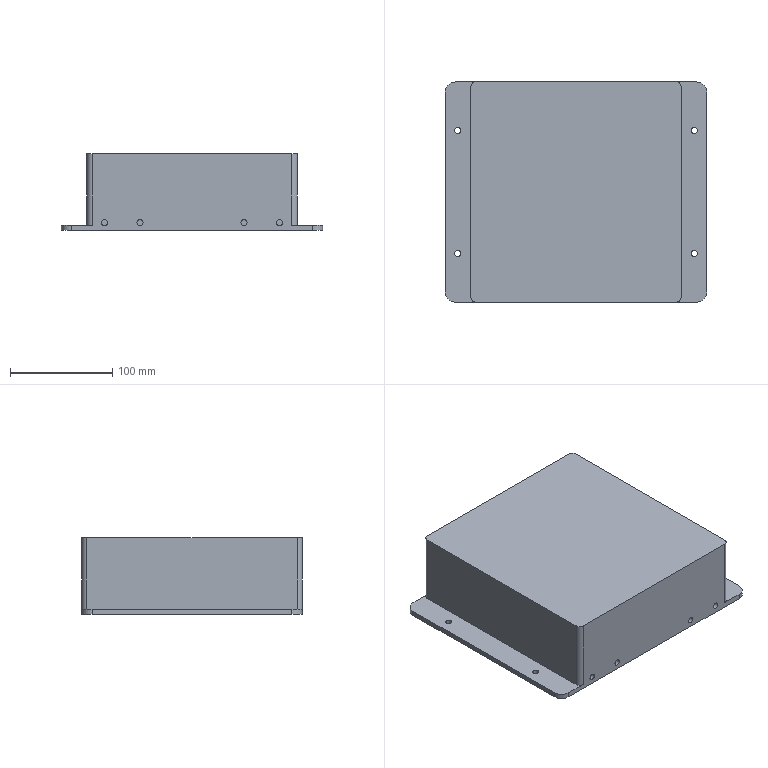NC program | NX | posted with a generic post | part box 255 x 215 x 75 mm
Lines 10479 to 11258 of 11258:
(ZLEVEL_PROFILE , TOOL : D6)
N20920 T12 M6
N20922 G54
N20924 G17 G0 G90 X-65.879 Y111.632 B0. C0. S9500 M3
N20926 G43 Z30. H12
N20928 Z0.507
N20930 G94 G1 Z-0.493 F1250.
N20932 X-66.701 Y111.156
N20934 G3 X-67. Y110.635 R0.6
N20936 G1 X-66.999 Y110.519
N20938 X-67. Y107.5
N20940 Y102.93
N20942 X-67.002 Y102.713
N20944 X-67. Y99.364
N20946 G3 X-66.699 Y98.845 R0.6
N20948 G1 X-65.878 Y98.372
N20950 Z0.507
N20952 G0 Z30.
N20954 X-64.122 Y98.371
N20956 Z0.507
N20958 G1 Z-0.493
N20960 X-63.3 Y98.845
N20962 G3 X-63. Y99.365 R0.6
N20964 G1 X-63.001 Y102.241
N20966 X-63. Y102.5
N20968 Y107.5
N20970 X-63.001 Y110.519
N20972 X-63. Y110.636
N20974 G3 X-63.298 Y111.157 R0.6
N20976 G1 X-64.12 Y111.636
N20978 Z0.507
N20980 G0 X-64.116 Y111.65 Z0.015
N20982 G1 Z-0.985
N20984 X-63.297 Y111.172
N20986 G2 X-63. Y110.651 R0.6
N20988 G1 X-63.001 Y110.519
N20990 Y107.846
N20992 X-63. Y107.5
N20994 Y102.5
N20996 X-63.001 Y102.241
N20998 Y99.481
N21000 X-63. Y99.35
N21002 G2 X-63.297 Y98.829 R0.6
N21004 G1 X-64.117 Y98.35
N21006 Z0.015
N21008 G0 Z30.
N21010 X-65.881 Y111.643
N21012 Z0.015
N21014 G1 Z-0.985
N21016 X-66.699 Y111.17
N21018 G3 X-66.999 Y110.65 R0.6
N21020 G1 Y107.846
N21022 X-67. Y107.5
N21024 Y102.93
N21026 X-67.002 Y102.713
N21028 X-66.999 Y99.349
N21030 G3 X-66.699 Y98.83 R0.6
N21032 G1 X-65.882 Y98.358
N21034 Z0.015
N21036 G0 X-65.885 Y98.345 Z-0.478
N21038 G1 Z-1.478
N21040 X-66.699 Y98.815
N21042 G2 X-66.999 Y99.334 R0.6
N21044 G1 X-67.002 Y102.713
N21046 X-67. Y102.93
N21048 Y107.5
N21050 X-66.999 Y107.846
N21052 Y110.666
N21054 G2 X-66.699 Y111.185 R0.6
N21056 G1 X-65.884 Y111.656
N21058 Z-0.478
N21060 G0 Z30.
N21062 X-64.113 Y98.336
N21064 Z-0.478
N21066 G1 Z-1.478
N21068 X-63.297 Y98.813
N21070 G3 X-63. Y99.335 R0.6
N21072 G1 X-63.001 Y99.481
N21074 Y102.241
N21076 X-63. Y102.5
N21078 Y107.5
N21080 X-63.001 Y107.846
N21082 Y110.519
N21084 X-63. Y110.666
N21086 G3 X-63.297 Y111.187 R0.6
N21088 G1 X-64.113 Y111.665
N21090 Z-0.478
N21092 G0 X-64.109 Y111.679 Z-0.97
N21094 G1 Z-1.97
N21096 X-63.297 Y111.203
N21098 G2 X-63. Y110.681 R0.6
N21100 G1 X-63.001 Y110.519
N21102 Y107.846
N21104 X-63. Y107.5
N21106 Y102.5
N21108 X-63.001 Y102.241
N21110 Y99.481
N21112 X-63. Y99.32
N21114 G2 X-63.297 Y98.798 R0.6
N21116 G1 X-64.11 Y98.322
N21118 Z-0.97
N21120 G0 Z30.
N21122 X-65.887 Y111.669
N21124 Z-0.97
N21126 G1 Z-1.97
N21128 X-66.699 Y111.2
N21130 G3 X-66.999 Y110.681 R0.6
N21132 G1 Y107.846
N21134 X-67. Y107.5
N21136 Y102.93
N21138 X-66.999 Y99.319
N21140 G3 X-66.699 Y98.799 R0.6
N21142 G1 X-65.888 Y98.331
N21144 Z-0.97
N21146 G0 X-65.891 Y98.318 Z-1.463
N21148 G1 Z-2.463
N21150 X-66.699 Y98.784
N21152 G2 X-66.999 Y99.304 R0.6
N21154 G1 X-67. Y102.93
N21156 Y107.5
N21158 X-66.998 Y107.846
N21160 X-66.999 Y110.696
N21162 G2 X-66.699 Y111.215 R0.6
N21164 G1 X-65.89 Y111.683
N21166 Z-1.463
N21168 G0 Z30.
N21170 X-64.106 Y98.308
N21172 Z-1.463
N21174 G1 Z-2.463
N21176 X-63.297 Y98.783
N21178 G3 X-63. Y99.305 R0.6
N21180 G1 X-63.002 Y99.481
N21182 Y102.241
N21184 X-63. Y102.5
N21186 Y107.5
N21188 X-63.002 Y107.846
N21190 Y110.519
N21192 X-63. Y110.696
N21194 G3 X-63.297 Y111.218 R0.6
N21196 G1 X-64.106 Y111.693
N21198 Z-1.463
N21200 G0 X-64.102 Y111.707 Z-1.956
N21202 G1 Z-2.956
N21204 X-63.296 Y111.233
N21206 G2 X-63. Y110.711 R0.6
N21208 G1 X-63.002 Y110.519
N21210 Y107.846
N21212 X-63. Y107.5
N21214 Y102.5
N21216 X-63.002 Y102.241
N21218 Y99.481
N21220 X-63. Y99.29
N21222 G2 X-63.296 Y98.768 R0.6
N21224 G1 X-64.103 Y98.294
N21226 Z-1.956
N21228 G0 Z30.
N21230 X-65.895 Y111.701
N21232 Z-1.956
N21234 G1 Z-2.956
N21236 X-66.701 Y111.232
N21238 G3 X-66.999 Y110.711 R0.6
N21240 G1 X-66.998 Y110.519
N21242 Y107.846
N21244 X-67. Y107.5
N21246 Y102.93
N21248 X-66.999 Y99.289
N21250 G3 X-66.699 Y98.769 R0.6
N21252 G1 X-65.894 Y98.305
N21254 Z-1.956
N21256 G0 X-65.897 Y98.292 Z-2.448
N21258 G1 Z-3.448
N21260 X-66.699 Y98.754
N21262 G2 X-66.999 Y99.273 R0.6
N21264 G1 X-67. Y102.93
N21266 Y107.5
N21268 X-66.998 Y107.846
N21270 Y110.519
N21272 X-66.999 Y110.726
N21274 G2 X-66.701 Y111.247 R0.6
N21276 G1 X-65.898 Y111.715
N21278 Z-2.448
N21280 G0 Z30.
N21282 X-64.099 Y98.28
N21284 Z-2.448
N21286 G1 Z-3.448
N21288 X-63.296 Y98.752
N21290 G3 X-63. Y99.275 R0.6
N21292 G1 X-63.002 Y99.481
N21294 Y102.241
N21296 X-63. Y102.5
N21298 Y107.5
N21300 X-63.002 Y107.846
N21302 Y110.519
N21304 X-63. Y110.726
N21306 G3 X-63.296 Y111.248 R0.6
N21308 G1 X-64.099 Y111.721
N21310 Z-2.448
N21312 G0 X-64.096 Y111.735 Z-2.941
N21314 G1 Z-3.941
N21316 X-63.296 Y111.264
N21318 G2 X-63. Y110.741 R0.6
N21320 G1 X-63.002 Y110.519
N21322 Y107.846
N21324 X-63. Y107.5
N21326 Y102.5
N21328 X-63.002 Y102.241
N21330 Y99.481
N21332 X-63. Y99.26
N21334 G2 X-63.296 Y98.737 R0.6
N21336 G1 X-64.096 Y98.266
N21338 Z-2.941
N21340 G0 Z30.
N21342 X-65.901 Y111.728
N21344 Z-2.941
N21346 G1 Z-3.941
N21348 X-66.701 Y111.262
N21350 G3 X-66.999 Y110.741 R0.6
N21352 G1 X-66.998 Y110.519
N21354 Y107.846
N21356 X-67. Y107.5
N21358 Y102.93
N21360 X-66.999 Y99.258
N21362 G3 X-66.698 Y98.739 R0.6
N21364 G1 X-65.901 Y98.279
N21366 Z-2.941
N21368 G0 X-65.904 Y98.265 Z-3.433
N21370 G1 Z-4.433
N21372 X-66.698 Y98.724
N21374 G2 X-66.999 Y99.243 R0.6
N21376 G1 X-67. Y102.93
N21378 Y107.5
N21380 X-66.998 Y107.835
N21382 X-66.999 Y110.756
N21384 G2 X-66.699 Y111.276 R0.6
N21386 G1 X-65.903 Y111.735
N21388 Z-3.433
N21390 G0 Z30.
N21392 X-64.092 Y98.252
N21394 Z-3.433
N21396 G1 Z-4.433
N21398 X-63.295 Y98.722
N21400 G3 X-63. Y99.245 R0.6
N21402 G1 X-63.003 Y99.481
N21404 Y102.241
N21406 X-63. Y102.5
N21408 Y107.5
N21410 X-63.001 Y107.835
N21412 X-63.003 Y110.519
N21414 X-63. Y110.757
N21416 G3 X-63.295 Y111.279 R0.6
N21418 G1 X-64.092 Y111.749
N21420 Z-3.433
N21422 G0 X-64.089 Y111.763 Z-3.926
N21424 G1 Z-4.926
N21426 X-63.295 Y111.294
N21428 G2 X-63. Y110.772 R0.6
N21430 G1 X-63.003 Y110.519
N21432 Y107.846
N21434 X-63. Y107.5
N21436 Y102.5
N21438 X-63.003 Y102.241
N21440 Y99.481
N21442 X-63. Y99.23
N21444 G2 X-63.295 Y98.707 R0.6
N21446 G1 X-64.089 Y98.238
N21448 Z-3.926
N21450 G0 Z30.
N21452 X-65.908 Y111.756
N21454 Z-3.926
N21456 G1 Z-4.926
N21458 X-66.701 Y111.292
N21460 G3 X-66.998 Y110.771 R0.6
N21462 G1 X-66.997 Y110.519
N21464 Y107.835
N21466 X-67. Y107.5
N21468 Y102.93
N21470 X-66.998 Y99.228
N21472 G3 X-66.698 Y98.709 R0.6
N21474 G1 X-65.907 Y98.252
N21476 Z-3.926
N21478 G0 X-65.862 Y98.236 Z-4.419
N21480 G1 Z-5.419
N21482 X-66.651 Y98.692
N21484 G2 X-66.95 Y99.212 R0.6
N21486 G3 X-66.982 Y102.67 R169.831
N21488 G1 Y107.414
N21490 G3 X-66.96 Y108.104 R13.816
N21492 G1 X-66.959 Y108.449
N21494 X-66.957 Y110.787
N21496 G2 X-66.656 Y111.307 R0.6
N21498 G1 X-65.87 Y111.759
N21500 Z-4.419
N21502 G0 Z30.
N21504 X-64.127 Y98.221
N21506 Z-4.419
N21508 G1 Z-5.419
N21510 X-63.337 Y98.69
N21512 G3 X-63.044 Y99.214 R0.6
N21514 G2 X-63.018 Y102.67 R84.586
N21516 G1 Y107.414
N21518 G2 X-63.05 Y110.788 R98.96
N21520 G3 X-63.346 Y111.31 R0.6
N21522 G1 X-64.136 Y111.774
N21524 Z-4.419
N21526 G0 X-64.221 Y111.77 Z-4.911
N21528 G1 Z-5.911
N21530 X-63.435 Y111.319
N21532 G2 X-63.134 Y110.8 R0.6
N21534 G1 X-63.129 Y108.449
N21536 X-63.089 Y107.328
N21538 X-63.084 Y107.285
N21540 Y102.715
N21542 G3 X-63.129 Y101.245 R24.84
N21544 G1 X-63.132 Y99.481
N21546 X-63.129 Y99.2
N21548 G2 X-63.424 Y98.678 R0.6
N21550 G1 X-64.211 Y98.213
N21552 Z-4.911
N21554 G0 Z30.
N21556 X-65.789 Y111.787
N21558 Z-4.911
N21560 G1 Z-5.911
N21562 X-66.576 Y111.322
N21564 G3 X-66.871 Y110.8 R0.6
N21566 G1 X-66.868 Y110.519
N21568 X-66.871 Y108.764
N21570 G2 X-66.916 Y107.285 R25.134
N21572 G1 Y102.715
N21574 X-66.911 Y102.672
N21576 X-66.871 Y101.551
N21578 X-66.866 Y99.2
N21580 G3 X-66.565 Y98.681 R0.6
N21582 G1 X-65.779 Y98.23
N21584 Z-4.911
N21586 G0 X-65.663 Y98.227 Z-5.404
N21588 G1 Z-6.404
N21590 X-66.449 Y98.681
N21592 G2 X-66.749 Y99.2 R0.6
N21594 G1 Y101.551
N21596 X-66.792 Y102.586
N21598 X-66.799 Y102.646
N21600 Y107.354
N21602 X-66.792 Y107.414
N21604 X-66.749 Y108.449
N21606 Y110.8
N21608 G2 X-66.449 Y111.32 R0.6
N21610 G1 X-65.664 Y111.773
N21612 Z-5.404
N21614 G0 Z30.
N21616 X-64.337 Y98.226
N21618 Z-5.404
N21620 G1 Z-6.404
N21622 X-63.551 Y98.681
N21624 G3 X-63.251 Y99.2 R0.6
N21626 G1 Y101.551
N21628 X-63.208 Y102.586
N21630 X-63.201 Y102.646
N21632 Y107.354
N21634 X-63.208 Y107.414
N21636 X-63.251 Y108.449
N21638 Y110.8
N21640 G3 X-63.551 Y111.32 R0.6
N21642 G1 X-64.337 Y111.774
N21644 Z-5.404
N21646 G0 X-64.509 Y111.773 Z-5.896
N21648 G1 Z-6.896
N21650 X-63.724 Y111.32
N21652 G2 X-63.424 Y110.8 R0.6
N21654 G1 Y108.449
N21656 X-63.374 Y107.414
N21658 Y102.651
N21660 X-63.424 Y101.551
N21662 Y99.2
N21664 G2 X-63.724 Y98.681 R0.6
N21666 G1 X-64.509 Y98.227
N21668 Z-5.896
N21670 G0 Z30.
N21672 X-65.491 Y111.773
N21674 Z-5.896
N21676 G1 Z-6.896
N21678 X-66.276 Y111.32
N21680 G3 X-66.576 Y110.8 R0.6
N21682 G1 Y108.449
N21684 X-66.626 Y107.414
N21686 Y102.651
N21688 X-66.576 Y101.551
N21690 Y99.2
N21692 G3 X-66.276 Y98.681 R0.6
N21694 G1 X-65.491 Y98.227
N21696 Z-5.896
N21698 G0 X-65.251 Y98.225 Z-6.389
N21700 G1 Z-7.389
N21702 X-66.041 Y98.681
N21704 G2 X-66.341 Y99.2 R0.6
N21706 G1 X-66.34 Y101.551
N21708 X-66.392 Y102.5
N21710 Y107.5
N21712 X-66.34 Y108.449
N21714 X-66.341 Y110.8
N21716 G2 X-66.041 Y111.32 R0.6
N21718 G1 X-65.251 Y111.775
N21720 Z-6.389
N21722 G0 Z30.
N21724 X-64.749 Y98.225
N21726 Z-6.389
N21728 G1 Z-7.389
N21730 X-63.959 Y98.681
N21732 G3 X-63.659 Y99.2 R0.6
N21734 G1 X-63.66 Y101.551
N21736 X-63.608 Y102.5
N21738 Y107.5
N21740 X-63.66 Y108.449
N21742 X-63.659 Y110.8
N21744 G3 X-63.959 Y111.32 R0.6
N21746 G1 X-64.749 Y111.775
N21748 Z-6.389
N21750 G0 X-65. Y111.976 Z-6.881
N21752 G1 Z-7.881
N21754 X-64.252 Y111.327
N21756 G2 X-63.965 Y110.8 R0.6
N21758 G3 X-63.914 Y107.414 R41.119
N21760 G1 Y102.93
N21762 G2 X-63.965 Y101.551 R38.767
N21764 G1 Y99.2
N21766 G2 X-64.265 Y98.681 R0.6
N21768 G1 X-65. Y98.023
N21770 Z-6.881
N21772 G0 Z30.
N21774 Y111.976
N21776 Z-6.881
N21778 G1 Z-7.881
N21780 X-65.749 Y111.328
N21782 G3 X-66.035 Y110.8 R0.6
N21784 G2 X-66.086 Y107.414 R39.521
N21786 G1 Y102.93
N21788 G3 X-66.035 Y101.551 R38.658
N21790 G1 Y99.2
N21792 G3 X-65.735 Y98.681 R0.6
N21794 G1 X-65. Y98.023
N21796 Z-6.881
N21798 G0 X-65.001 Y97.08 Z-7.374
N21800 G1 Z-8.374
N21802 X-65.318 Y98.681
N21804 G2 X-65.618 Y99.2 R0.6
N21806 G1 Y101.551
N21808 G3 X-65.69 Y102.5 R6.797
N21810 G1 Y107.5
N21812 G3 X-65.618 Y108.449 R6.797
N21814 G1 Y110.8
N21816 G2 X-65.318 Y111.32 R0.6
N21818 G1 X-65.001 Y112.921
N21820 Z-7.374
N21822 G0 Z30.
N21824 Y97.08
N21826 Z-7.374
N21828 G1 Z-8.374
N21830 X-64.656 Y98.67
N21832 G3 X-64.374 Y99.2 R0.6
N21834 G2 X-64.31 Y102.5 R30.274
N21836 G1 Y107.5
N21838 G2 X-64.374 Y110.8 R30.756
N21840 G3 X-64.656 Y111.33 R0.6
N21842 G1 X-65.001 Y112.921
N21844 Z-7.374
N21846 G0 X-65.002 Y113.645 Z-7.867
N21848 G1 Z-8.867
N21850 X-65.043 Y111.069
N21852 G2 X-64.902 Y110.805 R0.3
N21854 G3 X-64.83 Y107.443 R29.935
N21856 G1 Y102.557
N21858 X-64.837 Y102.541
N21860 X-64.902 Y101.551
N21862 Y99.195
N21864 G2 X-65.052 Y98.935 R0.3
N21866 G1 X-64.999 Y96.359
N21868 Z-7.867
N21870 G0 Z30.
N21872 X-65.002 Y113.645
N21874 Z-7.867
N21876 G1 Z-8.867
N21878 X-64.948 Y111.064
N21880 G3 X-65.098 Y110.804 R0.3
N21882 G1 Y108.449
N21884 X-65.163 Y107.459
N21886 X-65.17 Y107.443
N21888 Y102.557
N21890 G2 X-65.098 Y99.196 R29.944
N21892 G3 X-64.957 Y98.931 R0.3
N21894 G1 X-64.999 Y96.359
N21896 Z-7.867
N21898 G0 Z30.
N21900 M5
(FIXED_CONTOUR , TOOL : R3)
N21902 T17 M6
N21904 G54
N21906 G17 G0 G90 X-63.011 Y110.728 B0. C0. S9500 M3
N21908 G43 Z30. H17
N21910 Z1.2
N21912 G94 G1 Z-5.391 F2000.
N21914 Y110.654 Z-5.856
N21916 Y110.508 Z-6.303
N21918 X-63.01 Y110.294 Z-6.723
N21920 Y110.017 Z-7.103
N21922 Y109.684 Z-7.436
N21924 X-63.009 Y109.303 Z-7.713
N21926 Y108.884 Z-7.926
N21928 X-63.008 Y108.436 Z-8.071
N21930 Y107.971 Z-8.145
N21932 X-63.007 Y107.5 Z-8.144
N21934 X-63.005 Y105.705 Z-8.002
N21936 X-63.003 Y103.905 Z-8.007
N21938 Y103.372 Z-8.009
N21940 X-63.002 Y102.84 Z-8.013
N21942 X-63.007 Y102.5 Z-8.146
N21944 X-63.081 Z-8.534
N21946 X-63.093 Z-8.572
N21948 X-63.095 Y103.905 Z-8.577
N21950 X-63.097 Y105.705 Z-8.583
N21952 X-63.099 Y107.5 Z-8.59
N21954 X-63.151 Z-8.746
N21956 X-63.197 Z-8.842
N21958 X-63.195 Y105.704 Z-8.838
N21960 X-63.193 Y103.904 Z-8.833
N21962 X-63.191 Y102.5 Z-8.83
N21964 X-63.289 Z-9.017
N21966 X-63.29 Y103.904 Z-9.02
N21968 X-63.292 Y105.704 Z-9.023
N21970 X-63.294 Y107.5 Z-9.026
N21972 X-63.392 Z-9.178
N21974 X-63.39 Y105.704 Z-9.176
N21976 X-63.388 Y103.904 Z-9.173
N21978 X-63.386 Y102.5 Z-9.171
N21980 X-63.484 Z-9.289
N21982 X-63.485 Y103.904 Z-9.291
N21984 X-63.487 Y105.704 Z-9.294
N21986 X-63.49 Y107.5 Z-9.296
N21988 X-63.544 Z-9.362
N21990 X-63.587 Z-9.403
N21992 X-63.585 Y105.704 Z-9.401
N21994 X-63.583 Y103.904 Z-9.399
N21996 X-63.581 Y102.5 Z-9.398
N21998 X-63.679 Z-9.49
N22000 X-63.681 Y103.904 Z-9.491
N22002 X-63.683 Y105.704 Z-9.493
N22004 X-63.685 Y107.5 Z-9.495
N22006 X-63.782 Z-9.575
N22008 X-63.78 Y105.704 Z-9.574
N22010 X-63.778 Y103.904 Z-9.572
N22012 X-63.777 Y102.5 Z-9.571
N22014 X-63.874 Z-9.642
N22016 X-63.876 Y103.904 Z-9.643
N22018 X-63.878 Y105.704 Z-9.645
N22020 X-63.88 Y107.5 Z-9.646
N22022 X-63.978 Z-9.709
N22024 X-63.976 Y105.704 Z-9.708
N22026 X-63.973 Y103.904 Z-9.707
N22028 X-63.972 Y102.5 Z-9.706
N22030 X-64.069 Z-9.759
N22032 X-64.071 Y103.903 Z-9.76
N22034 X-64.073 Y105.703 Z-9.761
N22036 X-64.075 Y107.5 Z-9.763
N22038 X-64.173 Z-9.813
N22040 X-64.171 Y105.703 Z-9.812
N22042 X-64.169 Y103.903 Z-9.811
N22044 X-64.167 Y102.5
N22046 X-64.265 Z-9.849
N22048 X-64.266 Y103.903 Z-9.85
N22050 X-64.268 Y105.703 Z-9.851
N22052 X-64.27 Y107.5 Z-9.852
N22054 X-64.368 Z-9.89
N22056 X-64.366 Y105.703 Z-9.889
N22058 X-64.364 Y103.903
N22060 X-64.362 Y102.5 Z-9.888
N22062 X-64.46 Z-9.916
N22064 X-64.461 Y103.903
N22066 X-64.464 Y105.703 Z-9.917
N22068 X-64.466 Y107.5
N22070 X-64.563 Z-9.943
N22072 X-64.561 Y105.703 Z-9.942
N22074 X-64.559 Y103.903 Z-9.941
N22076 X-64.558 Y102.5
N22078 X-64.655 Z-9.962
N22080 X-64.657 Y103.903 Z-9.963
N22082 X-64.659 Y105.703
N22084 X-64.661 Y107.5
N22086 X-64.758 Z-9.975
N22088 X-64.756 Y105.703
N22090 X-64.754 Y103.903
N22092 X-64.753 Y102.5
N22094 X-64.85 Z-9.987
N22096 X-64.852 Y103.903
N22098 X-64.854 Y105.703 Z-9.988
N22100 X-64.856 Y107.5
N22102 X-64.954 Z-9.997
N22104 X-64.952 Y105.702
N22106 X-64.95 Y103.902
N22108 X-64.948 Y102.5
N22110 X-65. Z-9.999
N22112 X-65.046 Z-9.997
N22114 X-65.047 Y103.902
N22116 X-65.049 Y105.702
N22118 X-65.051 Y107.5
N22120 X-65.149 Z-9.987
N22122 X-65.147 Y105.702
N22124 X-65.145 Y103.902 Z-9.988
N22126 X-65.143 Y102.5
N22128 X-65.241 Z-9.976
N22130 X-65.242 Y103.902 Z-9.975
N22132 X-65.244 Y105.702
N22134 X-65.246 Y107.5
N22136 X-65.344 Z-9.962
N22138 X-65.342 Y105.702 Z-9.963
N22140 X-65.34 Y103.902
N22142 X-65.338 Y102.5
N22144 X-65.436 Z-9.943
N22146 X-65.438 Y103.902 Z-9.942
N22148 X-65.44 Y105.702
N22150 X-65.442 Y107.5 Z-9.941
N22152 X-65.539 Z-9.916
N22154 X-65.537 Y105.702 Z-9.917
N22156 X-65.535 Y103.902
N22158 X-65.534 Y102.5 Z-9.918
N22160 X-65.631 Z-9.891
N22162 X-65.633 Y103.902 Z-9.89
N22164 X-65.635 Y105.702 Z-9.889
N22166 X-65.637 Y107.5 Z-9.888
N22168 X-65.735 Z-9.85
N22170 X-65.732 Y105.702
N22172 X-65.73 Y103.902 Z-9.851
N22174 X-65.729 Y102.5 Z-9.852
N22176 X-65.826 Z-9.813
N22178 X-65.828 Y103.901
N22180 X-65.83 Y105.701 Z-9.812
N22182 X-65.832 Y107.5 Z-9.811
N22184 X-65.93 Z-9.76
N22186 X-65.928 Y105.701 Z-9.761
N22188 X-65.926 Y103.901 Z-9.762
N22190 X-65.924 Y102.5 Z-9.763
N22192 X-66.022 Z-9.709
N22194 X-66.023 Y103.901
N22196 X-66.025 Y105.701 Z-9.707
N22198 X-66.027 Y107.5 Z-9.706
N22200 X-66.125 Z-9.643
N22202 X-66.123 Y105.701 Z-9.644
N22204 X-66.121 Y103.901 Z-9.646
N22206 X-66.119 Y102.5 Z-9.647
N22208 X-66.217 Z-9.576
N22210 X-66.218 Y103.901 Z-9.575
N22212 X-66.22 Y105.701 Z-9.573
N22214 X-66.223 Y107.5 Z-9.572
N22216 X-66.32 Z-9.49
N22218 X-66.318 Y105.701 Z-9.492
N22220 X-66.316 Y103.901 Z-9.494
N22222 X-66.314 Y102.5 Z-9.496
N22224 X-66.412 Z-9.404
N22226 X-66.414 Y103.901 Z-9.403
N22228 X-66.416 Y105.701 Z-9.401
N22230 X-66.418 Y107.5 Z-9.399
N22232 X-66.456 Z-9.362
N22234 X-66.515 Z-9.29
N22236 X-66.513 Y105.701 Z-9.293
N22238 X-66.511 Y103.901 Z-9.295
N22240 X-66.51 Y102.5 Z-9.297
N22242 X-66.607 Z-9.179
N22244 X-66.609 Y103.901 Z-9.177
N22246 X-66.611 Y105.701 Z-9.175
N22248 X-66.613 Y107.5 Z-9.172
N22250 X-66.711 Z-9.019
N22252 X-66.709 Y105.7 Z-9.022
N22254 X-66.706 Y103.9 Z-9.025
N22256 X-66.705 Y102.5 Z-9.028
N22258 X-66.802 Z-8.844
N22260 X-66.804 Y103.9 Z-8.84
N22262 X-66.806 Y105.7 Z-8.836
N22264 X-66.808 Y107.5 Z-8.831
N22266 X-66.858 Z-8.72
N22268 X-66.906 Z-8.575
N22270 X-66.904 Y105.7 Z-8.581
N22272 X-66.902 Y103.9 Z-8.587
N22274 X-66.9 Y102.5 Z-8.592
N22276 X-66.924 Z-8.519
N22278 X-66.992 Z-8.149
N22280 X-66.993 Y102.85 Z-8.011
N22282 X-66.994 Y103.9 Z-8.009
N22284 X-66.996 Y105.7 Z-8.006
N22286 X-66.997 Y106.6 Z-8.046
N22288 X-66.998 Y107.5 Z-8.013
N22290 X-66.999 Y107.968 Z-7.959
N22292 Y108.421 Z-7.833
N22294 X-67. Y108.849 Z-7.637
N22296 Y109.241 Z-7.377
N22298 Y109.588 Z-7.058
N22300 X-67.001 Y109.881 Z-6.689
N22302 Y110.112 Z-6.279
N22304 Y110.276 Z-5.838
N22306 Y110.369 Z-5.377
N22308 Y110.389 Z-4.906
N22310 Z2.4
N22312 G0 Z30.
N22314 M5
(PLANAR_MILL_COPY_COPY_COPY_COPY_COPY , TOOL : D6A45)
N22316 T01 M6
N22318 G54
N22320 G17 G0 G90 X116.6 Y59.134 B0. C0. S9500 M3
N22322 G43 Z30. H1
N22324 Z0.
N22326 G94 G1 Z-1.5 F1250.
N22328 G3 X117.1 Y60. R1.
N22330 X115.5 Y61.6 R1.6
N22332 X117.1 Y60. R-1.6
N22334 X116.6 Y60.866 R1.
N22336 G1 Z0.
N22338 G0 Z30.
N22340 Y-60.866
N22342 Z0.
N22344 G1 Z-1.5
N22346 G3 X117.1 Y-60. R1.
N22348 X115.5 Y-58.4 R1.6
N22350 X117.1 Y-60. R-1.6
N22352 X116.6 Y-59.134 R1.
N22354 G1 Z0.
N22356 G0 Z30.
N22358 X0.866 Y-109.4
N22360 Z0.
N22362 G1 Z-1.5
N22364 G3 X0. Y-108.9 R1.
N22366 G1 X-117.5
N22368 G2 X-128.9 Y-97.5 R11.4
N22370 G1 Y97.5
N22372 G2 X-117.5 Y108.9 R11.4
N22374 G1 X-70.
N22376 G2 X-68.6 Y107.5 R1.4
N22378 G1 Y102.5
N22380 G2 X-70. Y101.1 R1.4
N22382 G1 X-92.5
N22384 G3 X-96.1 Y97.5 R3.6
N22386 G1 Y-97.5
N22388 G3 X-92.5 Y-101.1 R3.6
N22390 G1 X92.5
N22392 G3 X96.1 Y-97.5 R3.6
N22394 G1 Y97.5
N22396 G3 X92.5 Y101.1 R3.6
N22398 G1 X-60.
N22400 G2 X-61.4 Y102.5 R1.4
N22402 G1 Y107.5
N22404 G2 X-60. Y108.9 R1.4
N22406 G1 X117.5
N22408 G2 X128.9 Y97.5 R11.4
N22410 G1 Y-97.5
N22412 G2 X117.5 Y-108.9 R11.4
N22414 G1 X0.
N22416 G3 X-0.866 Y-109.4 R1.
N22418 G1 Z0.
N22420 G0 Z30.
N22422 X-116.6 Y-59.134
N22424 Z0.
N22426 G1 Z-1.5
N22428 G3 X-117.1 Y-60. R1.
N22430 X-115.5 Y-61.6 R1.6
N22432 X-117.1 Y-60. R-1.6
N22434 X-116.6 Y-60.866 R1.
N22436 G1 Z0.
N22438 G0 Z30.
N22440 Y60.866
N22442 Z0.
N22444 G1 Z-1.5
N22446 G3 X-117.1 Y60. R1.
N22448 X-115.5 Y58.4 R1.6
N22450 X-117.1 Y60. R-1.6
N22452 X-116.6 Y59.134 R1.
N22454 G1 Z0.
N22456 G0 Z30.
N22458 M5
N22460 M2